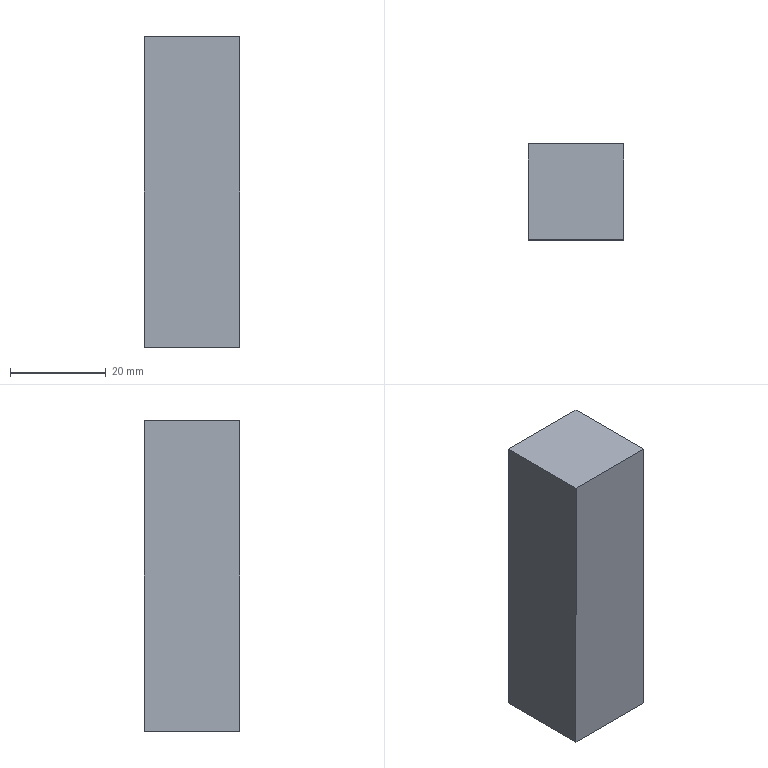Part | SolidWorks | features Extrusion 1 | 1 solid | 6 faces | box 20 x 20 x 65 mm | volume 26000 mm3 | plane 6
STEP:
#1=CARTESIAN_POINT('',(-10.,0.,-32.5));
#2=VERTEX_POINT('',#1);
#3=CARTESIAN_POINT('',(-10.,0.,32.5));
#4=VERTEX_POINT('',#3);
#5=CARTESIAN_POINT('',(-10.,0.,-32.5));
#6=DIRECTION('',(0.,0.,1.));
#7=VECTOR('',#6,1000.);
#8=LINE('',#5,#7);
#9=EDGE_CURVE('',#2,#4,#8,.T.);
#10=ORIENTED_EDGE('',*,*,#9,.T.);
#11=CARTESIAN_POINT('',(-10.,20.,32.5));
#12=VERTEX_POINT('',#11);
#13=CARTESIAN_POINT('',(-10.,20.,32.5));
#14=DIRECTION('',(0.,-1.,0.));
#15=VECTOR('',#14,1000.);
#16=LINE('',#13,#15);
#17=EDGE_CURVE('',#12,#4,#16,.T.);
#18=ORIENTED_EDGE('',*,*,#17,.F.);
#19=CARTESIAN_POINT('',(-10.,20.,-32.5));
#20=VERTEX_POINT('',#19);
#21=CARTESIAN_POINT('',(-10.,20.,-32.5));
#22=DIRECTION('',(0.,0.,1.));
#23=VECTOR('',#22,1000.);
#24=LINE('',#21,#23);
#25=EDGE_CURVE('',#20,#12,#24,.T.);
#26=ORIENTED_EDGE('',*,*,#25,.F.);
#27=CARTESIAN_POINT('',(-10.,20.,-32.5));
#28=DIRECTION('',(0.,-1.,0.));
#29=VECTOR('',#28,1000.);
#30=LINE('',#27,#29);
#31=EDGE_CURVE('',#20,#2,#30,.T.);
#32=ORIENTED_EDGE('',*,*,#31,.T.);
#33=EDGE_LOOP('',(#10,#18,#26,#32));
#34=FACE_OUTER_BOUND('',#33,.T.);
#35=CARTESIAN_POINT('',(-10.,20.,-32.5));
#36=DIRECTION('',(1.,0.,0.));
#37=DIRECTION('',(0.,0.,-1.));
#38=AXIS2_PLACEMENT_3D('',#35,#36,#37);
#39=PLANE('',#38);
#40=ADVANCED_FACE('',(#34),#39,.F.);
#41=CARTESIAN_POINT('',(10.,0.,32.5));
#42=VERTEX_POINT('',#41);
#43=CARTESIAN_POINT('',(-10.,0.,32.5));
#44=DIRECTION('',(1.,0.,0.));
#45=VECTOR('',#44,1000.);
#46=LINE('',#43,#45);
#47=EDGE_CURVE('',#4,#42,#46,.T.);
#48=ORIENTED_EDGE('',*,*,#47,.T.);
#49=CARTESIAN_POINT('',(10.,20.,32.5));
#50=VERTEX_POINT('',#49);
#51=CARTESIAN_POINT('',(10.,20.,32.5));
#52=DIRECTION('',(0.,-1.,0.));
#53=VECTOR('',#52,1000.);
#54=LINE('',#51,#53);
#55=EDGE_CURVE('',#50,#42,#54,.T.);
#56=ORIENTED_EDGE('',*,*,#55,.F.);
#57=CARTESIAN_POINT('',(-10.,20.,32.5));
#58=DIRECTION('',(1.,0.,0.));
#59=VECTOR('',#58,1000.);
#60=LINE('',#57,#59);
#61=EDGE_CURVE('',#12,#50,#60,.T.);
#62=ORIENTED_EDGE('',*,*,#61,.F.);
#63=ORIENTED_EDGE('',*,*,#17,.T.);
#64=EDGE_LOOP('',(#48,#56,#62,#63));
#65=FACE_OUTER_BOUND('',#64,.T.);
#66=CARTESIAN_POINT('',(-10.,20.,32.5));
#67=DIRECTION('',(0.,0.,-1.));
#68=DIRECTION('',(-1.,0.,0.));
#69=AXIS2_PLACEMENT_3D('',#66,#67,#68);
#70=PLANE('',#69);
#71=ADVANCED_FACE('',(#65),#70,.F.);
#72=CARTESIAN_POINT('',(10.,0.,-32.5));
#73=VERTEX_POINT('',#72);
#74=CARTESIAN_POINT('',(10.,0.,-32.5));
#75=DIRECTION('',(0.,0.,-1.));
#76=VECTOR('',#75,1000.);
#77=LINE('',#74,#76);
#78=EDGE_CURVE('',#42,#73,#77,.T.);
#79=ORIENTED_EDGE('',*,*,#78,.T.);
#80=CARTESIAN_POINT('',(10.,20.,-32.5));
#81=VERTEX_POINT('',#80);
#82=CARTESIAN_POINT('',(10.,20.,-32.5));
#83=DIRECTION('',(0.,-1.,0.));
#84=VECTOR('',#83,1000.);
#85=LINE('',#82,#84);
#86=EDGE_CURVE('',#81,#73,#85,.T.);
#87=ORIENTED_EDGE('',*,*,#86,.F.);
#88=CARTESIAN_POINT('',(10.,20.,-32.5));
#89=DIRECTION('',(0.,0.,-1.));
#90=VECTOR('',#89,1000.);
#91=LINE('',#88,#90);
#92=EDGE_CURVE('',#50,#81,#91,.T.);
#93=ORIENTED_EDGE('',*,*,#92,.F.);
#94=ORIENTED_EDGE('',*,*,#55,.T.);
#95=EDGE_LOOP('',(#79,#87,#93,#94));
#96=FACE_OUTER_BOUND('',#95,.T.);
#97=CARTESIAN_POINT('',(10.,20.,-32.5));
#98=DIRECTION('',(-1.,0.,0.));
#99=DIRECTION('',(0.,0.,1.));
#100=AXIS2_PLACEMENT_3D('',#97,#98,#99);
#101=PLANE('',#100);
#102=ADVANCED_FACE('',(#96),#101,.F.);
#103=CARTESIAN_POINT('',(-10.,0.,-32.5));
#104=DIRECTION('',(-1.,0.,0.));
#105=VECTOR('',#104,1000.);
#106=LINE('',#103,#105);
#107=EDGE_CURVE('',#73,#2,#106,.T.);
#108=ORIENTED_EDGE('',*,*,#107,.T.);
#109=ORIENTED_EDGE('',*,*,#31,.F.);
#110=CARTESIAN_POINT('',(-10.,20.,-32.5));
#111=DIRECTION('',(-1.,0.,0.));
#112=VECTOR('',#111,1000.);
#113=LINE('',#110,#112);
#114=EDGE_CURVE('',#81,#20,#113,.T.);
#115=ORIENTED_EDGE('',*,*,#114,.F.);
#116=ORIENTED_EDGE('',*,*,#86,.T.);
#117=EDGE_LOOP('',(#108,#109,#115,#116));
#118=FACE_OUTER_BOUND('',#117,.T.);
#119=CARTESIAN_POINT('',(-10.,20.,-32.5));
#120=DIRECTION('',(0.,0.,1.));
#121=DIRECTION('',(1.,0.,0.));
#122=AXIS2_PLACEMENT_3D('',#119,#120,#121);
#123=PLANE('',#122);
#124=ADVANCED_FACE('',(#118),#123,.F.);
#125=ORIENTED_EDGE('',*,*,#25,.T.);
#126=ORIENTED_EDGE('',*,*,#61,.T.);
#127=ORIENTED_EDGE('',*,*,#92,.T.);
#128=ORIENTED_EDGE('',*,*,#114,.T.);
#129=EDGE_LOOP('',(#125,#126,#127,#128));
#130=FACE_OUTER_BOUND('',#129,.T.);
#131=CARTESIAN_POINT('',(0.,20.,0.));
#132=DIRECTION('',(0.,1.,0.));
#133=DIRECTION('',(0.,0.,1.));
#134=AXIS2_PLACEMENT_3D('',#131,#132,#133);
#135=PLANE('',#134);
#136=ADVANCED_FACE('',(#130),#135,.T.);
#137=ORIENTED_EDGE('',*,*,#9,.F.);
#138=ORIENTED_EDGE('',*,*,#107,.F.);
#139=ORIENTED_EDGE('',*,*,#78,.F.);
#140=ORIENTED_EDGE('',*,*,#47,.F.);
#141=EDGE_LOOP('',(#137,#138,#139,#140));
#142=FACE_OUTER_BOUND('',#141,.T.);
#143=CARTESIAN_POINT('',(0.,0.,0.));
#144=DIRECTION('',(0.,1.,0.));
#145=DIRECTION('',(0.,0.,1.));
#146=AXIS2_PLACEMENT_3D('',#143,#144,#145);
#147=PLANE('',#146);
#148=ADVANCED_FACE('',(#142),#147,.F.);
#149=CLOSED_SHELL('',(#40,#71,#102,#124,#136,#148));
#150=MANIFOLD_SOLID_BREP('',#149);
#151=CARTESIAN_POINT('',(0.,0.,0.));
#152=DIRECTION('',(0.,0.,1.));
#153=DIRECTION('',(1.,0.,0.));
#154=AXIS2_PLACEMENT_3D('',#151,#152,#153);
#155=(LENGTH_UNIT()NAMED_UNIT(*)SI_UNIT(.MILLI.,.METRE.));
#156=UNCERTAINTY_MEASURE_WITH_UNIT(LENGTH_MEASURE(0.00001),#155,'','');
#157=(NAMED_UNIT(*)PLANE_ANGLE_UNIT()SI_UNIT($,.RADIAN.));
#158=(NAMED_UNIT(*)SI_UNIT($,.STERADIAN.)SOLID_ANGLE_UNIT());
#159=(GEOMETRIC_REPRESENTATION_CONTEXT(3)GLOBAL_UNCERTAINTY_ASSIGNED_CONTEXT((#156))GLOBAL_UNIT_ASSIGNED_CONTEXT((#155,#157,#158))REPRESENTATION_CONTEXT('',''));
#160=ADVANCED_BREP_SHAPE_REPRESENTATION('',(#150,#154),#159);